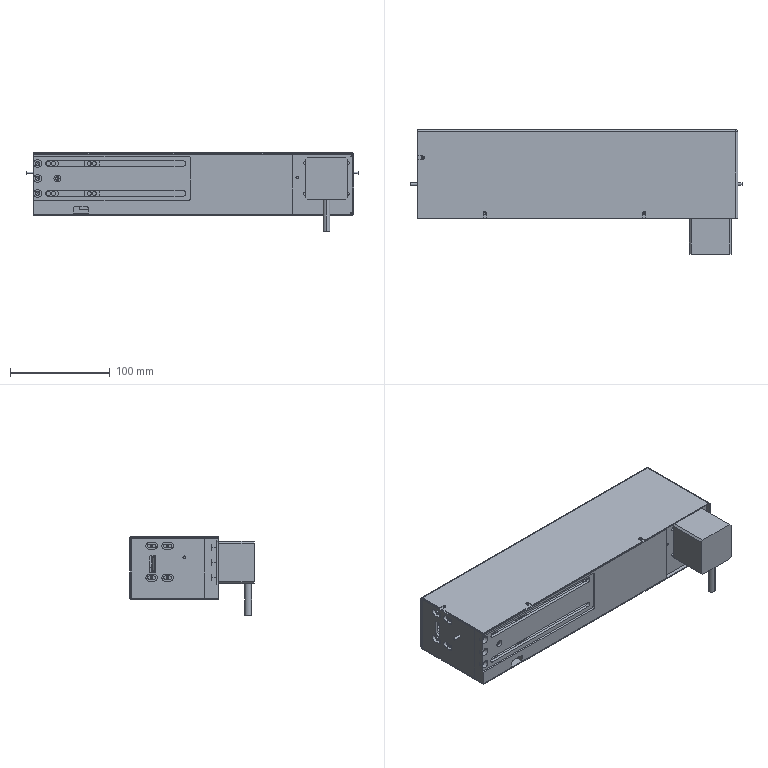Part | NX | features BREP 45 | 56 solids | 3151 faces | volume 570733 mm3 | cylinder 1379 | plane 991 | sphere 308 | cone 287 | torus 182 | spline 4 | commonest cylinder face diameters 2.5 x195 0.56 x126 0.3 x116 3.95 x112 6 x98 3.4 x88